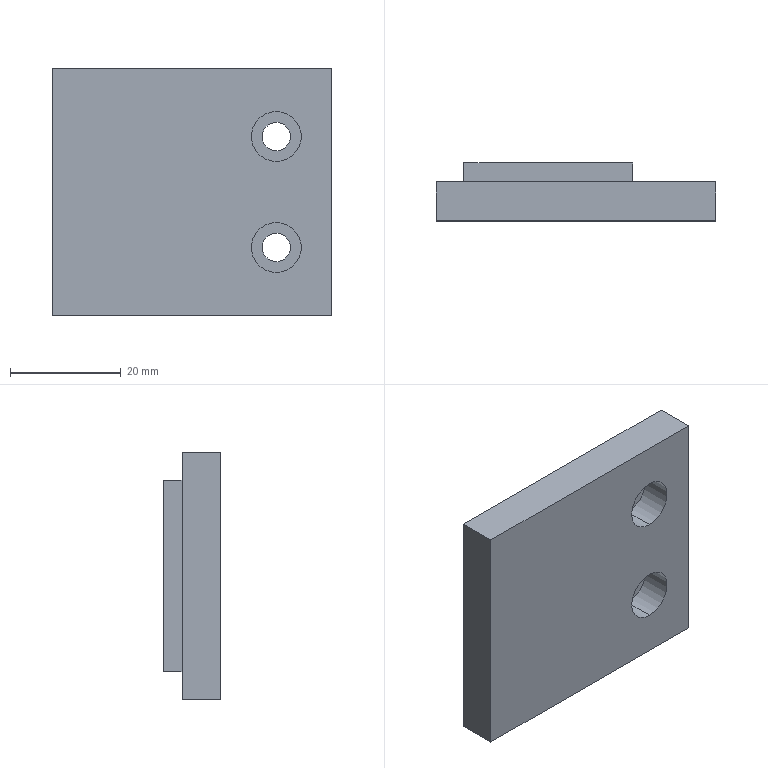Part | SolidWorks | features MoveFace 4, ICE 2, Cut 1, DelFace 1, SplitBody 1 | 1 solid | 21 faces | box 50.4 x 10.4 x 44.6 mm | volume 18550 mm3 | plane 13 | cylinder 8 | commonest cylinder face diameters 5.1 x4 9 x4
STEP:
#1=CARTESIAN_POINT('',(-20.,5.5,34.5));
#2=VERTEX_POINT('',#1);
#3=CARTESIAN_POINT('',(-20.,5.5,25.5));
#4=VERTEX_POINT('',#3);
#5=CARTESIAN_POINT('',(-20.,5.5,30.));
#6=DIRECTION('',(0.,-1.,0.));
#7=DIRECTION('',(0.,0.,-1.));
#8=AXIS2_PLACEMENT_3D('',#5,#6,#7);
#9=CIRCLE('',#8,4.5);
#10=EDGE_CURVE('',#2,#4,#9,.T.);
#11=ORIENTED_EDGE('',*,*,#10,.F.);
#12=CARTESIAN_POINT('',(-20.,0.,34.5));
#13=VERTEX_POINT('',#12);
#14=CARTESIAN_POINT('',(-20.,5.5,34.5));
#15=DIRECTION('',(0.,-1.,0.));
#16=VECTOR('',#15,1000.);
#17=LINE('',#14,#16);
#18=EDGE_CURVE('',#2,#13,#17,.T.);
#19=ORIENTED_EDGE('',*,*,#18,.T.);
#20=CARTESIAN_POINT('',(-20.,0.,25.5));
#21=VERTEX_POINT('',#20);
#22=CARTESIAN_POINT('',(-20.,0.,30.));
#23=DIRECTION('',(0.,-1.,0.));
#24=DIRECTION('',(0.,0.,-1.));
#25=AXIS2_PLACEMENT_3D('',#22,#23,#24);
#26=CIRCLE('',#25,4.5);
#27=EDGE_CURVE('',#13,#21,#26,.T.);
#28=ORIENTED_EDGE('',*,*,#27,.T.);
#29=CARTESIAN_POINT('',(-20.,5.5,25.5));
#30=DIRECTION('',(0.,-1.,0.));
#31=VECTOR('',#30,1000.);
#32=LINE('',#29,#31);
#33=EDGE_CURVE('',#4,#21,#32,.T.);
#34=ORIENTED_EDGE('',*,*,#33,.F.);
#35=EDGE_LOOP('',(#11,#19,#28,#34));
#36=FACE_OUTER_BOUND('',#35,.T.);
#37=CARTESIAN_POINT('',(-20.,5.5,30.));
#38=DIRECTION('',(0.,-1.,0.));
#39=DIRECTION('',(0.,0.,-1.));
#40=AXIS2_PLACEMENT_3D('',#37,#38,#39);
#41=CYLINDRICAL_SURFACE('',#40,4.5);
#42=ADVANCED_FACE('',(#36),#41,.F.);
#43=CARTESIAN_POINT('',(-20.,5.5,14.5));
#44=VERTEX_POINT('',#43);
#45=CARTESIAN_POINT('',(-20.,5.5,5.5));
#46=VERTEX_POINT('',#45);
#47=CARTESIAN_POINT('',(-20.,5.5,10.));
#48=DIRECTION('',(0.,-1.,0.));
#49=DIRECTION('',(0.,0.,1.));
#50=AXIS2_PLACEMENT_3D('',#47,#48,#49);
#51=CIRCLE('',#50,4.5);
#52=EDGE_CURVE('',#44,#46,#51,.T.);
#53=ORIENTED_EDGE('',*,*,#52,.F.);
#54=CARTESIAN_POINT('',(-20.,0.,14.5));
#55=VERTEX_POINT('',#54);
#56=CARTESIAN_POINT('',(-20.,5.5,14.5));
#57=DIRECTION('',(0.,-1.,0.));
#58=VECTOR('',#57,1000.);
#59=LINE('',#56,#58);
#60=EDGE_CURVE('',#44,#55,#59,.T.);
#61=ORIENTED_EDGE('',*,*,#60,.T.);
#62=CARTESIAN_POINT('',(-20.,0.,5.5));
#63=VERTEX_POINT('',#62);
#64=CARTESIAN_POINT('',(-20.,0.,10.));
#65=DIRECTION('',(0.,-1.,0.));
#66=DIRECTION('',(0.,0.,1.));
#67=AXIS2_PLACEMENT_3D('',#64,#65,#66);
#68=CIRCLE('',#67,4.5);
#69=EDGE_CURVE('',#55,#63,#68,.T.);
#70=ORIENTED_EDGE('',*,*,#69,.T.);
#71=CARTESIAN_POINT('',(-20.,5.5,5.5));
#72=DIRECTION('',(0.,-1.,0.));
#73=VECTOR('',#72,1000.);
#74=LINE('',#71,#73);
#75=EDGE_CURVE('',#46,#63,#74,.T.);
#76=ORIENTED_EDGE('',*,*,#75,.F.);
#77=EDGE_LOOP('',(#53,#61,#70,#76));
#78=FACE_OUTER_BOUND('',#77,.T.);
#79=CARTESIAN_POINT('',(-20.,5.5,10.));
#80=DIRECTION('',(0.,-1.,0.));
#81=DIRECTION('',(0.,0.,-1.));
#82=AXIS2_PLACEMENT_3D('',#79,#80,#81);
#83=CYLINDRICAL_SURFACE('',#82,4.5);
#84=ADVANCED_FACE('',(#78),#83,.F.);
#85=CARTESIAN_POINT('',(-22.55,5.5,10.));
#86=VERTEX_POINT('',#85);
#87=CARTESIAN_POINT('',(-17.45,5.5,10.));
#88=VERTEX_POINT('',#87);
#89=CARTESIAN_POINT('',(-20.,5.5,10.));
#90=DIRECTION('',(0.,-1.,0.));
#91=DIRECTION('',(0.,0.,1.));
#92=AXIS2_PLACEMENT_3D('',#89,#90,#91);
#93=CIRCLE('',#92,2.55);
#94=EDGE_CURVE('',#86,#88,#93,.T.);
#95=ORIENTED_EDGE('',*,*,#94,.T.);
#96=CARTESIAN_POINT('',(-17.45,7.,10.));
#97=VERTEX_POINT('',#96);
#98=CARTESIAN_POINT('',(-17.45,-5.6,10.));
#99=DIRECTION('',(0.,1.,0.));
#100=VECTOR('',#99,1000.);
#101=LINE('',#98,#100);
#102=EDGE_CURVE('',#88,#97,#101,.T.);
#103=ORIENTED_EDGE('',*,*,#102,.T.);
#104=CARTESIAN_POINT('',(-22.55,7.,10.));
#105=VERTEX_POINT('',#104);
#106=CARTESIAN_POINT('',(-20.,7.,10.));
#107=DIRECTION('',(0.,1.,0.));
#108=DIRECTION('',(1.,0.,0.));
#109=AXIS2_PLACEMENT_3D('',#106,#107,#108);
#110=CIRCLE('',#109,2.55);
#111=EDGE_CURVE('',#97,#105,#110,.T.);
#112=ORIENTED_EDGE('',*,*,#111,.T.);
#113=CARTESIAN_POINT('',(-22.55,-5.6,10.));
#114=DIRECTION('',(0.,1.,0.));
#115=VECTOR('',#114,1000.);
#116=LINE('',#113,#115);
#117=EDGE_CURVE('',#86,#105,#116,.T.);
#118=ORIENTED_EDGE('',*,*,#117,.F.);
#119=EDGE_LOOP('',(#95,#103,#112,#118));
#120=FACE_OUTER_BOUND('',#119,.T.);
#121=CARTESIAN_POINT('',(-20.,-5.6,10.));
#122=DIRECTION('',(0.,1.,0.));
#123=DIRECTION('',(-1.,0.,0.));
#124=AXIS2_PLACEMENT_3D('',#121,#122,#123);
#125=CYLINDRICAL_SURFACE('',#124,2.55);
#126=ADVANCED_FACE('',(#120),#125,.F.);
#127=CARTESIAN_POINT('',(-17.45,5.5,30.));
#128=VERTEX_POINT('',#127);
#129=CARTESIAN_POINT('',(-22.55,5.5,30.));
#130=VERTEX_POINT('',#129);
#131=CARTESIAN_POINT('',(-20.,5.5,30.));
#132=DIRECTION('',(0.,1.,0.));
#133=DIRECTION('',(0.,0.,-1.));
#134=AXIS2_PLACEMENT_3D('',#131,#132,#133);
#135=CIRCLE('',#134,2.55);
#136=EDGE_CURVE('',#128,#130,#135,.T.);
#137=ORIENTED_EDGE('',*,*,#136,.F.);
#138=CARTESIAN_POINT('',(-17.45,7.,30.));
#139=VERTEX_POINT('',#138);
#140=CARTESIAN_POINT('',(-17.45,-5.6,30.));
#141=DIRECTION('',(0.,1.,0.));
#142=VECTOR('',#141,1000.);
#143=LINE('',#140,#142);
#144=EDGE_CURVE('',#128,#139,#143,.T.);
#145=ORIENTED_EDGE('',*,*,#144,.T.);
#146=CARTESIAN_POINT('',(-22.55,7.,30.));
#147=VERTEX_POINT('',#146);
#148=CARTESIAN_POINT('',(-20.,7.,30.));
#149=DIRECTION('',(0.,1.,0.));
#150=DIRECTION('',(1.,0.,0.));
#151=AXIS2_PLACEMENT_3D('',#148,#149,#150);
#152=CIRCLE('',#151,2.55);
#153=EDGE_CURVE('',#139,#147,#152,.T.);
#154=ORIENTED_EDGE('',*,*,#153,.T.);
#155=CARTESIAN_POINT('',(-22.55,-5.6,30.));
#156=DIRECTION('',(0.,1.,0.));
#157=VECTOR('',#156,1000.);
#158=LINE('',#155,#157);
#159=EDGE_CURVE('',#130,#147,#158,.T.);
#160=ORIENTED_EDGE('',*,*,#159,.F.);
#161=EDGE_LOOP('',(#137,#145,#154,#160));
#162=FACE_OUTER_BOUND('',#161,.T.);
#163=CARTESIAN_POINT('',(-20.,-5.6,30.));
#164=DIRECTION('',(0.,1.,0.));
#165=DIRECTION('',(-1.,0.,0.));
#166=AXIS2_PLACEMENT_3D('',#163,#164,#165);
#167=CYLINDRICAL_SURFACE('',#166,2.55);
#168=ADVANCED_FACE('',(#162),#167,.F.);
#169=ORIENTED_EDGE('',*,*,#144,.F.);
#170=CARTESIAN_POINT('',(-20.,5.5,30.));
#171=DIRECTION('',(0.,1.,0.));
#172=DIRECTION('',(0.,0.,-1.));
#173=AXIS2_PLACEMENT_3D('',#170,#171,#172);
#174=CIRCLE('',#173,2.55);
#175=EDGE_CURVE('',#130,#128,#174,.T.);
#176=ORIENTED_EDGE('',*,*,#175,.F.);
#177=ORIENTED_EDGE('',*,*,#159,.T.);
#178=CARTESIAN_POINT('',(-20.,7.,30.));
#179=DIRECTION('',(0.,1.,0.));
#180=DIRECTION('',(1.,0.,0.));
#181=AXIS2_PLACEMENT_3D('',#178,#179,#180);
#182=CIRCLE('',#181,2.55);
#183=EDGE_CURVE('',#147,#139,#182,.T.);
#184=ORIENTED_EDGE('',*,*,#183,.T.);
#185=EDGE_LOOP('',(#169,#176,#177,#184));
#186=FACE_OUTER_BOUND('',#185,.T.);
#187=CARTESIAN_POINT('',(-20.,-5.6,30.));
#188=DIRECTION('',(0.,1.,0.));
#189=DIRECTION('',(-1.,0.,0.));
#190=AXIS2_PLACEMENT_3D('',#187,#188,#189);
#191=CYLINDRICAL_SURFACE('',#190,2.55);
#192=ADVANCED_FACE('',(#186),#191,.F.);
#193=CARTESIAN_POINT('',(-20.,0.,30.));
#194=DIRECTION('',(0.,-1.,0.));
#195=DIRECTION('',(0.,0.,-1.));
#196=AXIS2_PLACEMENT_3D('',#193,#194,#195);
#197=CIRCLE('',#196,4.5);
#198=EDGE_CURVE('',#21,#13,#197,.T.);
#199=ORIENTED_EDGE('',*,*,#198,.F.);
#200=ORIENTED_EDGE('',*,*,#27,.F.);
#201=EDGE_LOOP('',(#199,#200));
#202=FACE_BOUND('',#201,.T.);
#203=CARTESIAN_POINT('',(-20.,0.,10.));
#204=DIRECTION('',(0.,-1.,0.));
#205=DIRECTION('',(0.,0.,1.));
#206=AXIS2_PLACEMENT_3D('',#203,#204,#205);
#207=CIRCLE('',#206,4.5);
#208=EDGE_CURVE('',#63,#55,#207,.T.);
#209=ORIENTED_EDGE('',*,*,#208,.F.);
#210=ORIENTED_EDGE('',*,*,#69,.F.);
#211=EDGE_LOOP('',(#209,#210));
#212=FACE_BOUND('',#211,.T.);
#213=CARTESIAN_POINT('',(-10.,0.,42.3));
#214=VERTEX_POINT('',#213);
#215=CARTESIAN_POINT('',(-60.4,0.,42.3));
#216=VERTEX_POINT('',#215);
#217=CARTESIAN_POINT('',(-65.,0.,42.3));
#218=DIRECTION('',(-1.,0.,0.));
#219=VECTOR('',#218,1000.);
#220=LINE('',#217,#219);
#221=EDGE_CURVE('',#214,#216,#220,.T.);
#222=ORIENTED_EDGE('',*,*,#221,.T.);
#223=CARTESIAN_POINT('',(-60.4,0.,-2.3));
#224=VERTEX_POINT('',#223);
#225=CARTESIAN_POINT('',(-60.4,0.,2.3));
#226=DIRECTION('',(0.,0.,1.));
#227=VECTOR('',#226,1000.);
#228=LINE('',#225,#227);
#229=EDGE_CURVE('',#224,#216,#228,.T.);
#230=ORIENTED_EDGE('',*,*,#229,.F.);
#231=CARTESIAN_POINT('',(-10.,0.,-2.3));
#232=VERTEX_POINT('',#231);
#233=CARTESIAN_POINT('',(-65.,0.,-2.3));
#234=DIRECTION('',(1.,0.,0.));
#235=VECTOR('',#234,1000.);
#236=LINE('',#233,#235);
#237=EDGE_CURVE('',#224,#232,#236,.T.);
#238=ORIENTED_EDGE('',*,*,#237,.T.);
#239=CARTESIAN_POINT('',(-10.,0.,40.));
#240=DIRECTION('',(0.,0.,1.));
#241=VECTOR('',#240,1000.);
#242=LINE('',#239,#241);
#243=EDGE_CURVE('',#232,#214,#242,.T.);
#244=ORIENTED_EDGE('',*,*,#243,.T.);
#245=EDGE_LOOP('',(#222,#230,#238,#244));
#246=FACE_OUTER_BOUND('',#245,.T.);
#247=CARTESIAN_POINT('',(-65.,0.,40.));
#248=DIRECTION('',(0.,1.,0.));
#249=DIRECTION('',(0.,0.,1.));
#250=AXIS2_PLACEMENT_3D('',#247,#248,#249);
#251=PLANE('',#250);
#252=ADVANCED_FACE('',(#202,#212,#246),#251,.F.);
#253=CARTESIAN_POINT('',(-60.4,7.,42.3));
#254=VERTEX_POINT('',#253);
#255=CARTESIAN_POINT('',(-60.4,7.,42.3));
#256=DIRECTION('',(0.,1.,0.));
#257=VECTOR('',#256,1000.);
#258=LINE('',#255,#257);
#259=EDGE_CURVE('',#216,#254,#258,.T.);
#260=ORIENTED_EDGE('',*,*,#259,.T.);
#261=CARTESIAN_POINT('',(-60.4,7.,-2.3));
#262=VERTEX_POINT('',#261);
#263=CARTESIAN_POINT('',(-60.4,7.,2.3));
#264=DIRECTION('',(0.,0.,1.));
#265=VECTOR('',#264,1000.);
#266=LINE('',#263,#265);
#267=EDGE_CURVE('',#262,#254,#266,.T.);
#268=ORIENTED_EDGE('',*,*,#267,.F.);
#269=CARTESIAN_POINT('',(-60.4,7.,-2.3));
#270=DIRECTION('',(0.,1.,0.));
#271=VECTOR('',#270,1000.);
#272=LINE('',#269,#271);
#273=EDGE_CURVE('',#224,#262,#272,.T.);
#274=ORIENTED_EDGE('',*,*,#273,.F.);
#275=ORIENTED_EDGE('',*,*,#229,.T.);
#276=EDGE_LOOP('',(#260,#268,#274,#275));
#277=FACE_OUTER_BOUND('',#276,.T.);
#278=CARTESIAN_POINT('',(-60.4,7.,2.3));
#279=DIRECTION('',(1.,0.,0.));
#280=DIRECTION('',(0.,0.,-1.));
#281=AXIS2_PLACEMENT_3D('',#278,#279,#280);
#282=PLANE('',#281);
#283=ADVANCED_FACE('',(#277),#282,.F.);
#284=ORIENTED_EDGE('',*,*,#237,.F.);
#285=ORIENTED_EDGE('',*,*,#273,.T.);
#286=CARTESIAN_POINT('',(-10.,7.,-2.3));
#287=VERTEX_POINT('',#286);
#288=CARTESIAN_POINT('',(0.,7.,-2.3));
#289=DIRECTION('',(-1.,0.,0.));
#290=VECTOR('',#289,1000.);
#291=LINE('',#288,#290);
#292=EDGE_CURVE('',#287,#262,#291,.T.);
#293=ORIENTED_EDGE('',*,*,#292,.F.);
#294=CARTESIAN_POINT('',(-10.,-6.,-2.3));
#295=DIRECTION('',(0.,-1.,0.));
#296=VECTOR('',#295,1000.);
#297=LINE('',#294,#296);
#298=EDGE_CURVE('',#287,#232,#297,.T.);
#299=ORIENTED_EDGE('',*,*,#298,.T.);
#300=EDGE_LOOP('',(#284,#285,#293,#299));
#301=FACE_OUTER_BOUND('',#300,.T.);
#302=CARTESIAN_POINT('',(-65.,209.601,-2.3));
#303=DIRECTION('',(0.,0.,1.));
#304=DIRECTION('',(0.,-1.,0.));
#305=AXIS2_PLACEMENT_3D('',#302,#303,#304);
#306=PLANE('',#305);
#307=ADVANCED_FACE('',(#301),#306,.F.);
#308=ORIENTED_EDGE('',*,*,#298,.F.);
#309=CARTESIAN_POINT('',(-10.,7.,42.3));
#310=VERTEX_POINT('',#309);
#311=CARTESIAN_POINT('',(-10.,7.,40.));
#312=DIRECTION('',(0.,0.,-1.));
#313=VECTOR('',#312,1000.);
#314=LINE('',#311,#313);
#315=EDGE_CURVE('',#310,#287,#314,.T.);
#316=ORIENTED_EDGE('',*,*,#315,.F.);
#317=CARTESIAN_POINT('',(-10.,-6.,42.3));
#318=DIRECTION('',(0.,-1.,0.));
#319=VECTOR('',#318,1000.);
#320=LINE('',#317,#319);
#321=EDGE_CURVE('',#310,#214,#320,.T.);
#322=ORIENTED_EDGE('',*,*,#321,.T.);
#323=ORIENTED_EDGE('',*,*,#243,.F.);
#324=EDGE_LOOP('',(#308,#316,#322,#323));
#325=FACE_OUTER_BOUND('',#324,.T.);
#326=CARTESIAN_POINT('',(-10.,-6.,2.3));
#327=DIRECTION('',(-1.,0.,0.));
#328=DIRECTION('',(0.,0.,1.));
#329=AXIS2_PLACEMENT_3D('',#326,#327,#328);
#330=PLANE('',#329);
#331=ADVANCED_FACE('',(#325),#330,.F.);
#332=CARTESIAN_POINT('',(0.,7.,42.3));
#333=DIRECTION('',(1.,0.,0.));
#334=VECTOR('',#333,1000.);
#335=LINE('',#332,#334);
#336=EDGE_CURVE('',#254,#310,#335,.T.);
#337=ORIENTED_EDGE('',*,*,#336,.F.);
#338=ORIENTED_EDGE('',*,*,#259,.F.);
#339=ORIENTED_EDGE('',*,*,#221,.F.);
#340=ORIENTED_EDGE('',*,*,#321,.F.);
#341=EDGE_LOOP('',(#337,#338,#339,#340));
#342=FACE_OUTER_BOUND('',#341,.T.);
#343=CARTESIAN_POINT('',(-65.,209.601,42.3));
#344=DIRECTION('',(0.,0.,-1.));
#345=DIRECTION('',(0.,1.,0.));
#346=AXIS2_PLACEMENT_3D('',#343,#344,#345);
#347=PLANE('',#346);
#348=ADVANCED_FACE('',(#342),#347,.F.);
#349=CARTESIAN_POINT('',(-25.,10.4,2.7));
#350=VERTEX_POINT('',#349);
#351=CARTESIAN_POINT('',(-55.4,10.4,2.7));
#352=VERTEX_POINT('',#351);
#353=CARTESIAN_POINT('',(-25.,10.4,2.7));
#354=DIRECTION('',(-1.,0.,0.));
#355=VECTOR('',#354,1000.);
#356=LINE('',#353,#355);
#357=EDGE_CURVE('',#350,#352,#356,.T.);
#358=ORIENTED_EDGE('',*,*,#357,.F.);
#359=CARTESIAN_POINT('',(-25.,7.,2.7));
#360=VERTEX_POINT('',#359);
#361=CARTESIAN_POINT('',(-25.,14.,2.7));
#362=DIRECTION('',(0.,-1.,0.));
#363=VECTOR('',#362,1000.);
#364=LINE('',#361,#363);
#365=EDGE_CURVE('',#350,#360,#364,.T.);
#366=ORIENTED_EDGE('',*,*,#365,.T.);
#367=CARTESIAN_POINT('',(-55.4,7.,2.7));
#368=VERTEX_POINT('',#367);
#369=CARTESIAN_POINT('',(-65.,7.,2.7));
#370=DIRECTION('',(1.,0.,0.));
#371=VECTOR('',#370,1000.);
#372=LINE('',#369,#371);
#373=EDGE_CURVE('',#368,#360,#372,.T.);
#374=ORIENTED_EDGE('',*,*,#373,.F.);
#375=CARTESIAN_POINT('',(-55.4,14.,2.7));
#376=DIRECTION('',(0.,1.,0.));
#377=VECTOR('',#376,1000.);
#378=LINE('',#375,#377);
#379=EDGE_CURVE('',#368,#352,#378,.T.);
#380=ORIENTED_EDGE('',*,*,#379,.T.);
#381=EDGE_LOOP('',(#358,#366,#374,#380));
#382=FACE_OUTER_BOUND('',#381,.T.);
#383=CARTESIAN_POINT('',(-65.,14.,2.7));
#384=DIRECTION('',(0.,0.,1.));
#385=DIRECTION('',(0.,-1.,0.));
#386=AXIS2_PLACEMENT_3D('',#383,#384,#385);
#387=PLANE('',#386);
#388=ADVANCED_FACE('',(#382),#387,.F.);
#389=CARTESIAN_POINT('',(-25.,7.,37.3));
#390=VERTEX_POINT('',#389);
#391=CARTESIAN_POINT('',(-25.,7.,-2.3));
#392=DIRECTION('',(0.,0.,1.));
#393=VECTOR('',#392,1000.);
#394=LINE('',#391,#393);
#395=EDGE_CURVE('',#360,#390,#394,.T.);
#396=ORIENTED_EDGE('',*,*,#395,.T.);
#397=CARTESIAN_POINT('',(-55.4,7.,37.3));
#398=VERTEX_POINT('',#397);
#399=CARTESIAN_POINT('',(-65.,7.,37.3));
#400=DIRECTION('',(1.,0.,0.));
#401=VECTOR('',#400,1000.);
#402=LINE('',#399,#401);
#403=EDGE_CURVE('',#398,#390,#402,.T.);
#404=ORIENTED_EDGE('',*,*,#403,.F.);
#405=CARTESIAN_POINT('',(-55.4,7.,2.3));
#406=DIRECTION('',(0.,0.,1.));
#407=VECTOR('',#406,1000.);
#408=LINE('',#405,#407);
#409=EDGE_CURVE('',#368,#398,#408,.T.);
#410=ORIENTED_EDGE('',*,*,#409,.F.);
#411=ORIENTED_EDGE('',*,*,#373,.T.);
#412=EDGE_LOOP('',(#396,#404,#410,#411));
#413=FACE_BOUND('',#412,.T.);
#414=ORIENTED_EDGE('',*,*,#336,.T.);
#415=ORIENTED_EDGE('',*,*,#315,.T.);
#416=ORIENTED_EDGE('',*,*,#292,.T.);
#417=ORIENTED_EDGE('',*,*,#267,.T.);
#418=EDGE_LOOP('',(#414,#415,#416,#417));
#419=FACE_OUTER_BOUND('',#418,.T.);
#420=CARTESIAN_POINT('',(-20.,7.,10.));
#421=DIRECTION('',(0.,1.,0.));
#422=DIRECTION('',(1.,0.,0.));
#423=AXIS2_PLACEMENT_3D('',#420,#421,#422);
#424=CIRCLE('',#423,2.55);
#425=EDGE_CURVE('',#105,#97,#424,.T.);
#426=ORIENTED_EDGE('',*,*,#425,.F.);
#427=ORIENTED_EDGE('',*,*,#111,.F.);
#428=EDGE_LOOP('',(#426,#427));
#429=FACE_BOUND('',#428,.T.);
#430=ORIENTED_EDGE('',*,*,#183,.F.);
#431=ORIENTED_EDGE('',*,*,#153,.F.);
#432=EDGE_LOOP('',(#430,#431));
#433=FACE_BOUND('',#432,.T.);
#434=CARTESIAN_POINT('',(0.,7.,40.));
#435=DIRECTION('',(0.,-1.,0.));
#436=DIRECTION('',(1.,0.,0.));
#437=AXIS2_PLACEMENT_3D('',#434,#435,#436);
#438=PLANE('',#437);
#439=ADVANCED_FACE('',(#413,#419,#429,#433),#438,.F.);
#440=ORIENTED_EDGE('',*,*,#403,.T.);
#441=CARTESIAN_POINT('',(-25.,10.4,37.3));
#442=VERTEX_POINT('',#441);
#443=CARTESIAN_POINT('',(-25.,14.,37.3));
#444=DIRECTION('',(0.,1.,0.));
#445=VECTOR('',#444,1000.);
#446=LINE('',#443,#445);
#447=EDGE_CURVE('',#390,#442,#446,.T.);
#448=ORIENTED_EDGE('',*,*,#447,.T.);
#449=CARTESIAN_POINT('',(-55.4,10.4,37.3));
#450=VERTEX_POINT('',#449);
#451=CARTESIAN_POINT('',(-25.,10.4,37.3));
#452=DIRECTION('',(1.,0.,0.));
#453=VECTOR('',#452,1000.);
#454=LINE('',#451,#453);
#455=EDGE_CURVE('',#450,#442,#454,.T.);
#456=ORIENTED_EDGE('',*,*,#455,.F.);
#457=CARTESIAN_POINT('',(-55.4,14.,37.3));
#458=DIRECTION('',(0.,-1.,0.));
#459=VECTOR('',#458,1000.);
#460=LINE('',#457,#459);
#461=EDGE_CURVE('',#450,#398,#460,.T.);
#462=ORIENTED_EDGE('',*,*,#461,.T.);
#463=EDGE_LOOP('',(#440,#448,#456,#462));
#464=FACE_OUTER_BOUND('',#463,.T.);
#465=CARTESIAN_POINT('',(-65.,14.,37.3));
#466=DIRECTION('',(0.,0.,-1.));
#467=DIRECTION('',(-1.,0.,0.));
#468=AXIS2_PLACEMENT_3D('',#465,#466,#467);
#469=PLANE('',#468);
#470=ADVANCED_FACE('',(#464),#469,.F.);
#471=CARTESIAN_POINT('',(-55.4,10.4,2.3));
#472=DIRECTION('',(0.,0.,1.));
#473=VECTOR('',#472,1000.);
#474=LINE('',#471,#473);
#475=EDGE_CURVE('',#352,#450,#474,.T.);
#476=ORIENTED_EDGE('',*,*,#475,.F.);
#477=ORIENTED_EDGE('',*,*,#379,.F.);
#478=ORIENTED_EDGE('',*,*,#409,.T.);
#479=ORIENTED_EDGE('',*,*,#461,.F.);
#480=EDGE_LOOP('',(#476,#477,#478,#479));
#481=FACE_OUTER_BOUND('',#480,.T.);
#482=CARTESIAN_POINT('',(-55.4,10.4,2.3));
#483=DIRECTION('',(1.,0.,0.));
#484=DIRECTION('',(0.,0.,-1.));
#485=AXIS2_PLACEMENT_3D('',#482,#483,#484);
#486=PLANE('',#485);
#487=ADVANCED_FACE('',(#481),#486,.F.);
#488=CARTESIAN_POINT('',(-25.,10.4,-2.3));
#489=DIRECTION('',(0.,0.,1.));
#490=VECTOR('',#489,1000.);
#491=LINE('',#488,#490);
#492=EDGE_CURVE('',#350,#442,#491,.T.);
#493=ORIENTED_EDGE('',*,*,#492,.F.);
#494=ORIENTED_EDGE('',*,*,#357,.T.);
#495=ORIENTED_EDGE('',*,*,#475,.T.);
#496=ORIENTED_EDGE('',*,*,#455,.T.);
#497=EDGE_LOOP('',(#493,#494,#495,#496));
#498=FACE_OUTER_BOUND('',#497,.T.);
#499=CARTESIAN_POINT('',(-55.4,10.4,7.3));
#500=DIRECTION('',(0.,1.,0.));
#501=DIRECTION('',(-1.,0.,0.));
#502=AXIS2_PLACEMENT_3D('',#499,#500,#501);
#503=PLANE('',#502);
#504=ADVANCED_FACE('',(#498),#503,.T.);
#505=ORIENTED_EDGE('',*,*,#102,.F.);
#506=CARTESIAN_POINT('',(-20.,5.5,10.));
#507=DIRECTION('',(0.,-1.,0.));
#508=DIRECTION('',(0.,0.,1.));
#509=AXIS2_PLACEMENT_3D('',#506,#507,#508);
#510=CIRCLE('',#509,2.55);
#511=EDGE_CURVE('',#88,#86,#510,.T.);
#512=ORIENTED_EDGE('',*,*,#511,.T.);
#513=ORIENTED_EDGE('',*,*,#117,.T.);
#514=ORIENTED_EDGE('',*,*,#425,.T.);
#515=EDGE_LOOP('',(#505,#512,#513,#514));
#516=FACE_OUTER_BOUND('',#515,.T.);
#517=CARTESIAN_POINT('',(-20.,-5.6,10.));
#518=DIRECTION('',(0.,1.,0.));
#519=DIRECTION('',(-1.,0.,0.));
#520=AXIS2_PLACEMENT_3D('',#517,#518,#519);
#521=CYLINDRICAL_SURFACE('',#520,2.55);
#522=ADVANCED_FACE('',(#516),#521,.F.);
#523=CARTESIAN_POINT('',(-20.,5.5,10.));
#524=DIRECTION('',(0.,-1.,0.));
#525=DIRECTION('',(0.,0.,1.));
#526=AXIS2_PLACEMENT_3D('',#523,#524,#525);
#527=CIRCLE('',#526,4.5);
#528=EDGE_CURVE('',#46,#44,#527,.T.);
#529=ORIENTED_EDGE('',*,*,#528,.T.);
#530=ORIENTED_EDGE('',*,*,#52,.T.);
#531=EDGE_LOOP('',(#529,#530));
#532=FACE_OUTER_BOUND('',#531,.T.);
#533=ORIENTED_EDGE('',*,*,#94,.F.);
#534=ORIENTED_EDGE('',*,*,#511,.F.);
#535=EDGE_LOOP('',(#533,#534));
#536=FACE_BOUND('',#535,.T.);
#537=CARTESIAN_POINT('',(-20.,5.5,10.));
#538=DIRECTION('',(0.,1.,0.));
#539=DIRECTION('',(0.,0.,1.));
#540=AXIS2_PLACEMENT_3D('',#537,#538,#539);
#541=PLANE('',#540);
#542=ADVANCED_FACE('',(#532,#536),#541,.F.);
#543=ORIENTED_EDGE('',*,*,#60,.F.);
#544=ORIENTED_EDGE('',*,*,#528,.F.);
#545=ORIENTED_EDGE('',*,*,#75,.T.);
#546=ORIENTED_EDGE('',*,*,#208,.T.);
#547=EDGE_LOOP('',(#543,#544,#545,#546));
#548=FACE_OUTER_BOUND('',#547,.T.);
#549=CARTESIAN_POINT('',(-20.,5.5,10.));
#550=DIRECTION('',(0.,-1.,0.));
#551=DIRECTION('',(0.,0.,-1.));
#552=AXIS2_PLACEMENT_3D('',#549,#550,#551);
#553=CYLINDRICAL_SURFACE('',#552,4.5);
#554=ADVANCED_FACE('',(#548),#553,.F.);
#555=CARTESIAN_POINT('',(-20.,5.5,30.));
#556=DIRECTION('',(0.,-1.,0.));
#557=DIRECTION('',(0.,0.,-1.));
#558=AXIS2_PLACEMENT_3D('',#555,#556,#557);
#559=CIRCLE('',#558,4.5);
#560=EDGE_CURVE('',#4,#2,#559,.T.);
#561=ORIENTED_EDGE('',*,*,#560,.T.);
#562=ORIENTED_EDGE('',*,*,#10,.T.);
#563=EDGE_LOOP('',(#561,#562));
#564=FACE_OUTER_BOUND('',#563,.T.);
#565=ORIENTED_EDGE('',*,*,#175,.T.);
#566=ORIENTED_EDGE('',*,*,#136,.T.);
#567=EDGE_LOOP('',(#565,#566));
#568=FACE_BOUND('',#567,.T.);
#569=CARTESIAN_POINT('',(-20.,5.5,30.));
#570=DIRECTION('',(0.,-1.,0.));
#571=DIRECTION('',(0.,0.,-1.));
#572=AXIS2_PLACEMENT_3D('',#569,#570,#571);
#573=PLANE('',#572);
#574=ADVANCED_FACE('',(#564,#568),#573,.T.);
#575=ORIENTED_EDGE('',*,*,#18,.F.);
#576=ORIENTED_EDGE('',*,*,#560,.F.);
#577=ORIENTED_EDGE('',*,*,#33,.T.);
#578=ORIENTED_EDGE('',*,*,#198,.T.);
#579=EDGE_LOOP('',(#575,#576,#577,#578));
#580=FACE_OUTER_BOUND('',#579,.T.);
#581=CARTESIAN_POINT('',(-20.,5.5,30.));
#582=DIRECTION('',(0.,-1.,0.));
#583=DIRECTION('',(0.,0.,-1.));
#584=AXIS2_PLACEMENT_3D('',#581,#582,#583);
#585=CYLINDRICAL_SURFACE('',#584,4.5);
#586=ADVANCED_FACE('',(#580),#585,.F.);
#587=ORIENTED_EDGE('',*,*,#492,.T.);
#588=ORIENTED_EDGE('',*,*,#447,.F.);
#589=ORIENTED_EDGE('',*,*,#395,.F.);
#590=ORIENTED_EDGE('',*,*,#365,.F.);
#591=EDGE_LOOP('',(#587,#588,#589,#590));
#592=FACE_OUTER_BOUND('',#591,.T.);
#593=CARTESIAN_POINT('',(-25.,-40.055,-2.3));
#594=DIRECTION('',(-1.,0.,0.));
#595=DIRECTION('',(0.,-1.,0.));
#596=AXIS2_PLACEMENT_3D('',#593,#594,#595);
#597=PLANE('',#596);
#598=ADVANCED_FACE('',(#592),#597,.F.);
#599=CLOSED_SHELL('',(#42,#84,#126,#168,#192,#252,#283,#307,#331,#348,#388,#439,#470,#487,#504,#522,#542,#554,#574,#586,#598));
#600=MANIFOLD_SOLID_BREP('',#599);
#601=CARTESIAN_POINT('',(0.,0.,0.));
#602=DIRECTION('',(0.,0.,1.));
#603=DIRECTION('',(1.,0.,0.));
#604=AXIS2_PLACEMENT_3D('',#601,#602,#603);
#605=(LENGTH_UNIT()NAMED_UNIT(*)SI_UNIT(.MILLI.,.METRE.));
#606=UNCERTAINTY_MEASURE_WITH_UNIT(LENGTH_MEASURE(0.00001),#605,'','');
#607=(NAMED_UNIT(*)PLANE_ANGLE_UNIT()SI_UNIT($,.RADIAN.));
#608=(NAMED_UNIT(*)SI_UNIT($,.STERADIAN.)SOLID_ANGLE_UNIT());
#609=(GEOMETRIC_REPRESENTATION_CONTEXT(3)GLOBAL_UNCERTAINTY_ASSIGNED_CONTEXT((#606))GLOBAL_UNIT_ASSIGNED_CONTEXT((#605,#607,#608))REPRESENTATION_CONTEXT('',''));
#610=ADVANCED_BREP_SHAPE_REPRESENTATION('',(#600,#604),#609);